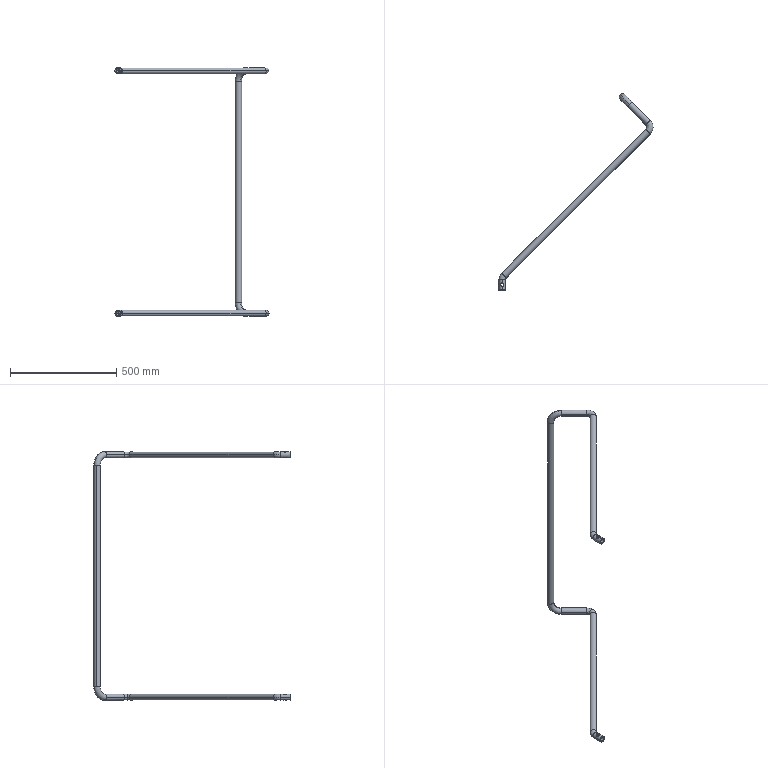Part | SolidWorks | features 3DProfileFeature 3, Cut 1, Shell 1, Sweep 1 | 1 solid | 66 faces | box 724.68 x 923.528 x 1170 mm | volume 1404787 mm3 | cylinder 36 | torus 28 | plane 2 | commonest cylinder face diameters 20 x14 30 x14 16.386 x8